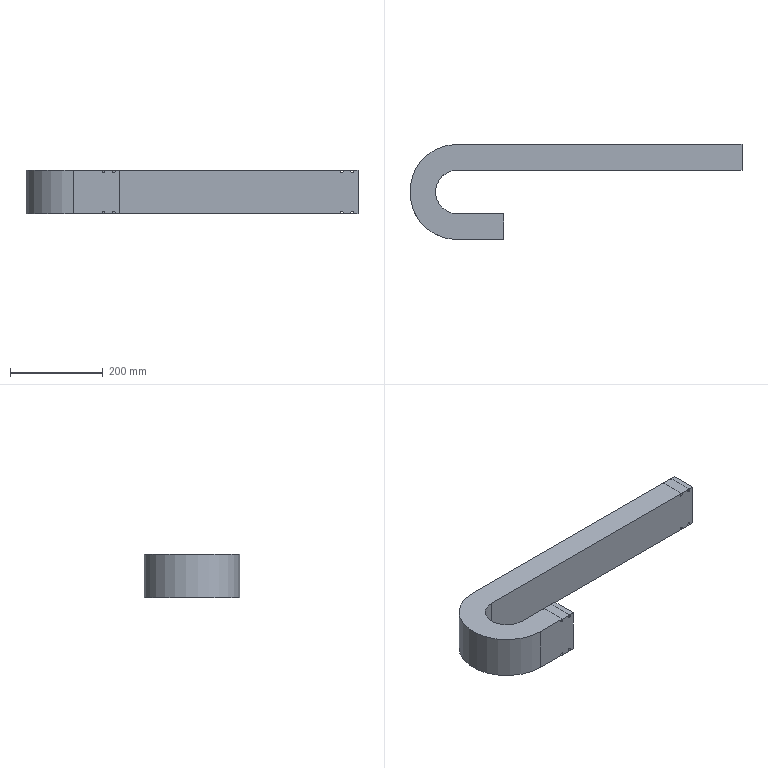Part | NX | 1 solid | 26 faces | box 718 x 206 x 95 mm | volume 1837118 mm3 | plane 14 | cylinder 12 | commonest cylinder face diameters 5.8 x8 94 x1 105 x1 195 x1 206 x1
STEP:
#1=CARTESIAN_POINT('',(0.,22.5,37.5));
#2=VERTEX_POINT('',#1);
#3=CARTESIAN_POINT('',(0.,22.5,-37.5));
#4=VERTEX_POINT('',#3);
#5=CARTESIAN_POINT('',(0.,22.5,37.5));
#6=DIRECTION('',(0.,0.,-1.));
#7=VECTOR('',#6,1000.);
#8=LINE('',#5,#7);
#9=EDGE_CURVE('',#2,#4,#8,.T.);
#10=ORIENTED_EDGE('',*,*,#9,.T.);
#11=CARTESIAN_POINT('',(100.,22.5,-37.5));
#12=VERTEX_POINT('',#11);
#13=CARTESIAN_POINT('',(0.,22.5,-37.5));
#14=DIRECTION('',(1.,0.,0.));
#15=VECTOR('',#14,1000.);
#16=LINE('',#13,#15);
#17=EDGE_CURVE('',#4,#12,#16,.T.);
#18=ORIENTED_EDGE('',*,*,#17,.T.);
#19=CARTESIAN_POINT('',(100.,22.5,37.5));
#20=VERTEX_POINT('',#19);
#21=CARTESIAN_POINT('',(100.,22.5,37.5));
#22=DIRECTION('',(0.,0.,-1.));
#23=VECTOR('',#22,1000.);
#24=LINE('',#21,#23);
#25=EDGE_CURVE('',#20,#12,#24,.T.);
#26=ORIENTED_EDGE('',*,*,#25,.F.);
#27=CARTESIAN_POINT('',(0.,22.5,37.5));
#28=DIRECTION('',(1.,0.,0.));
#29=VECTOR('',#28,1000.);
#30=LINE('',#27,#29);
#31=EDGE_CURVE('',#2,#20,#30,.T.);
#32=ORIENTED_EDGE('',*,*,#31,.F.);
#33=EDGE_LOOP('',(#10,#18,#26,#32));
#34=FACE_BOUND('',#33,.T.);
#35=CARTESIAN_POINT('',(0.,22.5,37.5));
#36=DIRECTION('',(0.,-1.,0.));
#37=DIRECTION('',(0.,0.,-1.));
#38=AXIS2_PLACEMENT_3D('',#35,#36,#37);
#39=PLANE('',#38);
#40=ADVANCED_FACE('',(#34),#39,.T.);
#41=CARTESIAN_POINT('',(0.,-22.5,-37.5));
#42=VERTEX_POINT('',#41);
#43=CARTESIAN_POINT('',(0.,-22.5,37.5));
#44=VERTEX_POINT('',#43);
#45=CARTESIAN_POINT('',(0.,-22.5,37.5));
#46=DIRECTION('',(0.,0.,1.));
#47=VECTOR('',#46,1000.);
#48=LINE('',#45,#47);
#49=EDGE_CURVE('',#42,#44,#48,.T.);
#50=ORIENTED_EDGE('',*,*,#49,.T.);
#51=CARTESIAN_POINT('',(100.,-22.5,37.5));
#52=VERTEX_POINT('',#51);
#53=CARTESIAN_POINT('',(0.,-22.5,37.5));
#54=DIRECTION('',(1.,0.,0.));
#55=VECTOR('',#54,1000.);
#56=LINE('',#53,#55);
#57=EDGE_CURVE('',#44,#52,#56,.T.);
#58=ORIENTED_EDGE('',*,*,#57,.T.);
#59=CARTESIAN_POINT('',(100.,-22.5,-37.5));
#60=VERTEX_POINT('',#59);
#61=CARTESIAN_POINT('',(100.,-22.5,37.5));
#62=DIRECTION('',(0.,0.,1.));
#63=VECTOR('',#62,1000.);
#64=LINE('',#61,#63);
#65=EDGE_CURVE('',#60,#52,#64,.T.);
#66=ORIENTED_EDGE('',*,*,#65,.F.);
#67=CARTESIAN_POINT('',(0.,-22.5,-37.5));
#68=DIRECTION('',(1.,0.,0.));
#69=VECTOR('',#68,1000.);
#70=LINE('',#67,#69);
#71=EDGE_CURVE('',#42,#60,#70,.T.);
#72=ORIENTED_EDGE('',*,*,#71,.F.);
#73=EDGE_LOOP('',(#50,#58,#66,#72));
#74=FACE_BOUND('',#73,.T.);
#75=CARTESIAN_POINT('',(0.,-22.5,37.5));
#76=DIRECTION('',(0.,1.,0.));
#77=DIRECTION('',(0.,0.,1.));
#78=AXIS2_PLACEMENT_3D('',#75,#76,#77);
#79=PLANE('',#78);
#80=ADVANCED_FACE('',(#74),#79,.T.);
#81=CARTESIAN_POINT('',(65.,28.,47.4));
#82=VERTEX_POINT('',#81);
#83=CARTESIAN_POINT('',(65.,28.,44.5));
#84=DIRECTION('',(0.,1.,0.));
#85=DIRECTION('',(0.,0.,1.));
#86=AXIS2_PLACEMENT_3D('',#83,#84,#85);
#87=CIRCLE('',#86,2.9);
#88=EDGE_CURVE('',#82,#82,#87,.T.);
#89=ORIENTED_EDGE('',*,*,#88,.F.);
#90=EDGE_LOOP('',(#89));
#91=FACE_BOUND('',#90,.T.);
#92=CARTESIAN_POINT('',(65.,28.,-41.6));
#93=VERTEX_POINT('',#92);
#94=CARTESIAN_POINT('',(65.,28.,-44.5));
#95=DIRECTION('',(0.,1.,0.));
#96=DIRECTION('',(0.,0.,1.));
#97=AXIS2_PLACEMENT_3D('',#94,#95,#96);
#98=CIRCLE('',#97,2.9);
#99=EDGE_CURVE('',#93,#93,#98,.T.);
#100=ORIENTED_EDGE('',*,*,#99,.F.);
#101=EDGE_LOOP('',(#100));
#102=FACE_BOUND('',#101,.T.);
#103=CARTESIAN_POINT('',(87.5,28.,41.6));
#104=VERTEX_POINT('',#103);
#105=CARTESIAN_POINT('',(87.5,28.,44.5));
#106=DIRECTION('',(0.,1.,0.));
#107=DIRECTION('',(0.,0.,-1.));
#108=AXIS2_PLACEMENT_3D('',#105,#106,#107);
#109=CIRCLE('',#108,2.9);
#110=EDGE_CURVE('',#104,#104,#109,.T.);
#111=ORIENTED_EDGE('',*,*,#110,.F.);
#112=EDGE_LOOP('',(#111));
#113=FACE_BOUND('',#112,.T.);
#114=CARTESIAN_POINT('',(87.5,28.,-41.6));
#115=VERTEX_POINT('',#114);
#116=CARTESIAN_POINT('',(87.5,28.,-44.5));
#117=DIRECTION('',(0.,1.,0.));
#118=DIRECTION('',(0.,0.,1.));
#119=AXIS2_PLACEMENT_3D('',#116,#117,#118);
#120=CIRCLE('',#119,2.9);
#121=EDGE_CURVE('',#115,#115,#120,.T.);
#122=ORIENTED_EDGE('',*,*,#121,.F.);
#123=EDGE_LOOP('',(#122));
#124=FACE_BOUND('',#123,.T.);
#125=CARTESIAN_POINT('',(0.,28.,47.5));
#126=VERTEX_POINT('',#125);
#127=CARTESIAN_POINT('',(0.,28.,-47.5));
#128=VERTEX_POINT('',#127);
#129=CARTESIAN_POINT('',(0.,28.,47.5));
#130=DIRECTION('',(0.,0.,-1.));
#131=VECTOR('',#130,1000.);
#132=LINE('',#129,#131);
#133=EDGE_CURVE('',#126,#128,#132,.T.);
#134=ORIENTED_EDGE('',*,*,#133,.F.);
#135=CARTESIAN_POINT('',(100.,28.,47.5));
#136=VERTEX_POINT('',#135);
#137=CARTESIAN_POINT('',(0.,28.,47.5));
#138=DIRECTION('',(1.,0.,0.));
#139=VECTOR('',#138,1000.);
#140=LINE('',#137,#139);
#141=EDGE_CURVE('',#126,#136,#140,.T.);
#142=ORIENTED_EDGE('',*,*,#141,.T.);
#143=CARTESIAN_POINT('',(100.,28.,-47.5));
#144=VERTEX_POINT('',#143);
#145=CARTESIAN_POINT('',(100.,28.,47.5));
#146=DIRECTION('',(0.,0.,-1.));
#147=VECTOR('',#146,1000.);
#148=LINE('',#145,#147);
#149=EDGE_CURVE('',#136,#144,#148,.T.);
#150=ORIENTED_EDGE('',*,*,#149,.T.);
#151=CARTESIAN_POINT('',(0.,28.,-47.5));
#152=DIRECTION('',(1.,0.,0.));
#153=VECTOR('',#152,1000.);
#154=LINE('',#151,#153);
#155=EDGE_CURVE('',#128,#144,#154,.T.);
#156=ORIENTED_EDGE('',*,*,#155,.F.);
#157=EDGE_LOOP('',(#134,#142,#150,#156));
#158=FACE_BOUND('',#157,.T.);
#159=CARTESIAN_POINT('',(0.,28.,47.5));
#160=DIRECTION('',(0.,-1.,0.));
#161=DIRECTION('',(0.,0.,-1.));
#162=AXIS2_PLACEMENT_3D('',#159,#160,#161);
#163=PLANE('',#162);
#164=ADVANCED_FACE('',(#91,#102,#113,#124,#158),#163,.F.);
#165=CARTESIAN_POINT('',(65.,-28.,47.4));
#166=VERTEX_POINT('',#165);
#167=CARTESIAN_POINT('',(65.,-28.,44.5));
#168=DIRECTION('',(0.,1.,0.));
#169=DIRECTION('',(0.,0.,1.));
#170=AXIS2_PLACEMENT_3D('',#167,#168,#169);
#171=CIRCLE('',#170,2.9);
#172=EDGE_CURVE('',#166,#166,#171,.T.);
#173=ORIENTED_EDGE('',*,*,#172,.T.);
#174=EDGE_LOOP('',(#173));
#175=FACE_BOUND('',#174,.T.);
#176=CARTESIAN_POINT('',(65.,-28.,-41.6));
#177=VERTEX_POINT('',#176);
#178=CARTESIAN_POINT('',(65.,-28.,-44.5));
#179=DIRECTION('',(0.,1.,0.));
#180=DIRECTION('',(0.,0.,1.));
#181=AXIS2_PLACEMENT_3D('',#178,#179,#180);
#182=CIRCLE('',#181,2.9);
#183=EDGE_CURVE('',#177,#177,#182,.T.);
#184=ORIENTED_EDGE('',*,*,#183,.T.);
#185=EDGE_LOOP('',(#184));
#186=FACE_BOUND('',#185,.T.);
#187=CARTESIAN_POINT('',(87.5,-28.,41.6));
#188=VERTEX_POINT('',#187);
#189=CARTESIAN_POINT('',(87.5,-28.,44.5));
#190=DIRECTION('',(0.,1.,0.));
#191=DIRECTION('',(0.,0.,-1.));
#192=AXIS2_PLACEMENT_3D('',#189,#190,#191);
#193=CIRCLE('',#192,2.9);
#194=EDGE_CURVE('',#188,#188,#193,.T.);
#195=ORIENTED_EDGE('',*,*,#194,.T.);
#196=EDGE_LOOP('',(#195));
#197=FACE_BOUND('',#196,.T.);
#198=CARTESIAN_POINT('',(87.5,-28.,-41.6));
#199=VERTEX_POINT('',#198);
#200=CARTESIAN_POINT('',(87.5,-28.,-44.5));
#201=DIRECTION('',(0.,1.,0.));
#202=DIRECTION('',(0.,0.,1.));
#203=AXIS2_PLACEMENT_3D('',#200,#201,#202);
#204=CIRCLE('',#203,2.9);
#205=EDGE_CURVE('',#199,#199,#204,.T.);
#206=ORIENTED_EDGE('',*,*,#205,.T.);
#207=EDGE_LOOP('',(#206));
#208=FACE_BOUND('',#207,.T.);
#209=CARTESIAN_POINT('',(0.,-28.,-47.5));
#210=VERTEX_POINT('',#209);
#211=CARTESIAN_POINT('',(0.,-28.,47.5));
#212=VERTEX_POINT('',#211);
#213=CARTESIAN_POINT('',(0.,-28.,47.5));
#214=DIRECTION('',(0.,0.,1.));
#215=VECTOR('',#214,1000.);
#216=LINE('',#213,#215);
#217=EDGE_CURVE('',#210,#212,#216,.T.);
#218=ORIENTED_EDGE('',*,*,#217,.F.);
#219=CARTESIAN_POINT('',(100.,-28.,-47.5));
#220=VERTEX_POINT('',#219);
#221=CARTESIAN_POINT('',(0.,-28.,-47.5));
#222=DIRECTION('',(1.,0.,0.));
#223=VECTOR('',#222,1000.);
#224=LINE('',#221,#223);
#225=EDGE_CURVE('',#210,#220,#224,.T.);
#226=ORIENTED_EDGE('',*,*,#225,.T.);
#227=CARTESIAN_POINT('',(100.,-28.,47.5));
#228=VERTEX_POINT('',#227);
#229=CARTESIAN_POINT('',(100.,-28.,47.5));
#230=DIRECTION('',(0.,0.,1.));
#231=VECTOR('',#230,1000.);
#232=LINE('',#229,#231);
#233=EDGE_CURVE('',#220,#228,#232,.T.);
#234=ORIENTED_EDGE('',*,*,#233,.T.);
#235=CARTESIAN_POINT('',(0.,-28.,47.5));
#236=DIRECTION('',(1.,0.,0.));
#237=VECTOR('',#236,1000.);
#238=LINE('',#235,#237);
#239=EDGE_CURVE('',#212,#228,#238,.T.);
#240=ORIENTED_EDGE('',*,*,#239,.F.);
#241=EDGE_LOOP('',(#218,#226,#234,#240));
#242=FACE_BOUND('',#241,.T.);
#243=CARTESIAN_POINT('',(0.,-28.,47.5));
#244=DIRECTION('',(0.,1.,0.));
#245=DIRECTION('',(0.,0.,1.));
#246=AXIS2_PLACEMENT_3D('',#243,#244,#245);
#247=PLANE('',#246);
#248=ADVANCED_FACE('',(#175,#186,#197,#208,#242),#247,.F.);
#249=CARTESIAN_POINT('',(0.,127.5,37.5));
#250=VERTEX_POINT('',#249);
#251=CARTESIAN_POINT('',(0.,127.5,-37.5));
#252=VERTEX_POINT('',#251);
#253=CARTESIAN_POINT('',(0.,127.5,37.5));
#254=DIRECTION('',(0.,0.,-1.));
#255=VECTOR('',#254,1000.);
#256=LINE('',#253,#255);
#257=EDGE_CURVE('',#250,#252,#256,.T.);
#258=ORIENTED_EDGE('',*,*,#257,.T.);
#259=CARTESIAN_POINT('',(0.,75.,-37.5));
#260=DIRECTION('',(0.,0.,1.));
#261=DIRECTION('',(1.,0.,0.));
#262=AXIS2_PLACEMENT_3D('',#259,#260,#261);
#263=CIRCLE('',#262,52.5);
#264=EDGE_CURVE('',#252,#4,#263,.T.);
#265=ORIENTED_EDGE('',*,*,#264,.T.);
#266=ORIENTED_EDGE('',*,*,#9,.F.);
#267=CARTESIAN_POINT('',(0.,75.,37.5));
#268=DIRECTION('',(0.,0.,1.));
#269=DIRECTION('',(1.,0.,0.));
#270=AXIS2_PLACEMENT_3D('',#267,#268,#269);
#271=CIRCLE('',#270,52.5);
#272=EDGE_CURVE('',#250,#2,#271,.T.);
#273=ORIENTED_EDGE('',*,*,#272,.F.);
#274=EDGE_LOOP('',(#258,#265,#266,#273));
#275=FACE_BOUND('',#274,.T.);
#276=CARTESIAN_POINT('',(0.,75.,0.));
#277=DIRECTION('',(0.,0.,1.));
#278=DIRECTION('',(1.,0.,0.));
#279=AXIS2_PLACEMENT_3D('',#276,#277,#278);
#280=CYLINDRICAL_SURFACE('',#279,52.5);
#281=ADVANCED_FACE('',(#275),#280,.T.);
#282=CARTESIAN_POINT('',(0.,172.5,-37.5));
#283=VERTEX_POINT('',#282);
#284=CARTESIAN_POINT('',(0.,172.5,37.5));
#285=VERTEX_POINT('',#284);
#286=CARTESIAN_POINT('',(0.,172.5,37.5));
#287=DIRECTION('',(0.,0.,1.));
#288=VECTOR('',#287,1000.);
#289=LINE('',#286,#288);
#290=EDGE_CURVE('',#283,#285,#289,.T.);
#291=ORIENTED_EDGE('',*,*,#290,.T.);
#292=CARTESIAN_POINT('',(0.,75.,37.5));
#293=DIRECTION('',(0.,0.,1.));
#294=DIRECTION('',(1.,0.,0.));
#295=AXIS2_PLACEMENT_3D('',#292,#293,#294);
#296=CIRCLE('',#295,97.5);
#297=EDGE_CURVE('',#285,#44,#296,.T.);
#298=ORIENTED_EDGE('',*,*,#297,.T.);
#299=ORIENTED_EDGE('',*,*,#49,.F.);
#300=CARTESIAN_POINT('',(0.,75.,-37.5));
#301=DIRECTION('',(0.,0.,1.));
#302=DIRECTION('',(1.,0.,0.));
#303=AXIS2_PLACEMENT_3D('',#300,#301,#302);
#304=CIRCLE('',#303,97.5);
#305=EDGE_CURVE('',#283,#42,#304,.T.);
#306=ORIENTED_EDGE('',*,*,#305,.F.);
#307=EDGE_LOOP('',(#291,#298,#299,#306));
#308=FACE_BOUND('',#307,.T.);
#309=CARTESIAN_POINT('',(0.,75.,0.));
#310=DIRECTION('',(0.,0.,1.));
#311=DIRECTION('',(1.,0.,0.));
#312=AXIS2_PLACEMENT_3D('',#309,#310,#311);
#313=CYLINDRICAL_SURFACE('',#312,97.5);
#314=ADVANCED_FACE('',(#308),#313,.F.);
#315=CARTESIAN_POINT('',(0.,122.,47.5));
#316=VERTEX_POINT('',#315);
#317=CARTESIAN_POINT('',(0.,122.,-47.5));
#318=VERTEX_POINT('',#317);
#319=CARTESIAN_POINT('',(0.,122.,47.5));
#320=DIRECTION('',(0.,0.,-1.));
#321=VECTOR('',#320,1000.);
#322=LINE('',#319,#321);
#323=EDGE_CURVE('',#316,#318,#322,.T.);
#324=ORIENTED_EDGE('',*,*,#323,.F.);
#325=CARTESIAN_POINT('',(0.,75.,47.5));
#326=DIRECTION('',(0.,0.,1.));
#327=DIRECTION('',(1.,0.,0.));
#328=AXIS2_PLACEMENT_3D('',#325,#326,#327);
#329=CIRCLE('',#328,47.);
#330=EDGE_CURVE('',#316,#126,#329,.T.);
#331=ORIENTED_EDGE('',*,*,#330,.T.);
#332=ORIENTED_EDGE('',*,*,#133,.T.);
#333=CARTESIAN_POINT('',(0.,75.,-47.5));
#334=DIRECTION('',(0.,0.,1.));
#335=DIRECTION('',(1.,0.,0.));
#336=AXIS2_PLACEMENT_3D('',#333,#334,#335);
#337=CIRCLE('',#336,47.);
#338=EDGE_CURVE('',#318,#128,#337,.T.);
#339=ORIENTED_EDGE('',*,*,#338,.F.);
#340=EDGE_LOOP('',(#324,#331,#332,#339));
#341=FACE_BOUND('',#340,.T.);
#342=CARTESIAN_POINT('',(0.,75.,0.));
#343=DIRECTION('',(0.,0.,1.));
#344=DIRECTION('',(1.,0.,0.));
#345=AXIS2_PLACEMENT_3D('',#342,#343,#344);
#346=CYLINDRICAL_SURFACE('',#345,47.);
#347=ADVANCED_FACE('',(#341),#346,.F.);
#348=CARTESIAN_POINT('',(0.,178.,-47.5));
#349=VERTEX_POINT('',#348);
#350=CARTESIAN_POINT('',(0.,178.,47.5));
#351=VERTEX_POINT('',#350);
#352=CARTESIAN_POINT('',(0.,178.,47.5));
#353=DIRECTION('',(0.,0.,1.));
#354=VECTOR('',#353,1000.);
#355=LINE('',#352,#354);
#356=EDGE_CURVE('',#349,#351,#355,.T.);
#357=ORIENTED_EDGE('',*,*,#356,.F.);
#358=CARTESIAN_POINT('',(0.,75.,-47.5));
#359=DIRECTION('',(0.,0.,1.));
#360=DIRECTION('',(1.,0.,0.));
#361=AXIS2_PLACEMENT_3D('',#358,#359,#360);
#362=CIRCLE('',#361,103.);
#363=EDGE_CURVE('',#349,#210,#362,.T.);
#364=ORIENTED_EDGE('',*,*,#363,.T.);
#365=ORIENTED_EDGE('',*,*,#217,.T.);
#366=CARTESIAN_POINT('',(0.,75.,47.5));
#367=DIRECTION('',(0.,0.,1.));
#368=DIRECTION('',(1.,0.,0.));
#369=AXIS2_PLACEMENT_3D('',#366,#367,#368);
#370=CIRCLE('',#369,103.);
#371=EDGE_CURVE('',#351,#212,#370,.T.);
#372=ORIENTED_EDGE('',*,*,#371,.F.);
#373=EDGE_LOOP('',(#357,#364,#365,#372));
#374=FACE_BOUND('',#373,.T.);
#375=CARTESIAN_POINT('',(0.,75.,0.));
#376=DIRECTION('',(0.,0.,1.));
#377=DIRECTION('',(1.,0.,0.));
#378=AXIS2_PLACEMENT_3D('',#375,#376,#377);
#379=CYLINDRICAL_SURFACE('',#378,103.);
#380=ADVANCED_FACE('',(#374),#379,.T.);
#381=CARTESIAN_POINT('',(615.,172.5,37.5));
#382=VERTEX_POINT('',#381);
#383=CARTESIAN_POINT('',(615.,127.5,37.5));
#384=VERTEX_POINT('',#383);
#385=CARTESIAN_POINT('',(615.,127.5,37.5));
#386=DIRECTION('',(0.,-1.,0.));
#387=VECTOR('',#386,1000.);
#388=LINE('',#385,#387);
#389=EDGE_CURVE('',#382,#384,#388,.T.);
#390=ORIENTED_EDGE('',*,*,#389,.T.);
#391=CARTESIAN_POINT('',(0.,127.5,37.5));
#392=DIRECTION('',(1.,0.,0.));
#393=VECTOR('',#392,1000.);
#394=LINE('',#391,#393);
#395=EDGE_CURVE('',#250,#384,#394,.T.);
#396=ORIENTED_EDGE('',*,*,#395,.F.);
#397=ORIENTED_EDGE('',*,*,#272,.T.);
#398=ORIENTED_EDGE('',*,*,#31,.T.);
#399=CARTESIAN_POINT('',(100.,22.5,37.5));
#400=DIRECTION('',(0.,1.,0.));
#401=VECTOR('',#400,1000.);
#402=LINE('',#399,#401);
#403=EDGE_CURVE('',#52,#20,#402,.T.);
#404=ORIENTED_EDGE('',*,*,#403,.F.);
#405=ORIENTED_EDGE('',*,*,#57,.F.);
#406=ORIENTED_EDGE('',*,*,#297,.F.);
#407=CARTESIAN_POINT('',(0.,172.5,37.5));
#408=DIRECTION('',(1.,0.,0.));
#409=VECTOR('',#408,1000.);
#410=LINE('',#407,#409);
#411=EDGE_CURVE('',#285,#382,#410,.T.);
#412=ORIENTED_EDGE('',*,*,#411,.T.);
#413=EDGE_LOOP('',(#390,#396,#397,#398,#404,#405,#406,#412));
#414=FACE_BOUND('',#413,.T.);
#415=CARTESIAN_POINT('',(0.,127.5,37.5));
#416=DIRECTION('',(0.,0.,1.));
#417=DIRECTION('',(1.,0.,0.));
#418=AXIS2_PLACEMENT_3D('',#415,#416,#417);
#419=PLANE('',#418);
#420=ADVANCED_FACE('',(#414),#419,.F.);
#421=CARTESIAN_POINT('',(615.,127.5,-37.5));
#422=VERTEX_POINT('',#421);
#423=CARTESIAN_POINT('',(615.,127.5,37.5));
#424=DIRECTION('',(0.,0.,-1.));
#425=VECTOR('',#424,1000.);
#426=LINE('',#423,#425);
#427=EDGE_CURVE('',#384,#422,#426,.T.);
#428=ORIENTED_EDGE('',*,*,#427,.T.);
#429=CARTESIAN_POINT('',(0.,127.5,-37.5));
#430=DIRECTION('',(1.,0.,0.));
#431=VECTOR('',#430,1000.);
#432=LINE('',#429,#431);
#433=EDGE_CURVE('',#252,#422,#432,.T.);
#434=ORIENTED_EDGE('',*,*,#433,.F.);
#435=ORIENTED_EDGE('',*,*,#257,.F.);
#436=ORIENTED_EDGE('',*,*,#395,.T.);
#437=EDGE_LOOP('',(#428,#434,#435,#436));
#438=FACE_BOUND('',#437,.T.);
#439=CARTESIAN_POINT('',(0.,127.5,37.5));
#440=DIRECTION('',(0.,-1.,0.));
#441=DIRECTION('',(1.,0.,0.));
#442=AXIS2_PLACEMENT_3D('',#439,#440,#441);
#443=PLANE('',#442);
#444=ADVANCED_FACE('',(#438),#443,.F.);
#445=CARTESIAN_POINT('',(615.,172.5,-37.5));
#446=VERTEX_POINT('',#445);
#447=CARTESIAN_POINT('',(615.,127.5,-37.5));
#448=DIRECTION('',(0.,1.,0.));
#449=VECTOR('',#448,1000.);
#450=LINE('',#447,#449);
#451=EDGE_CURVE('',#422,#446,#450,.T.);
#452=ORIENTED_EDGE('',*,*,#451,.T.);
#453=CARTESIAN_POINT('',(0.,172.5,-37.5));
#454=DIRECTION('',(1.,0.,0.));
#455=VECTOR('',#454,1000.);
#456=LINE('',#453,#455);
#457=EDGE_CURVE('',#283,#446,#456,.T.);
#458=ORIENTED_EDGE('',*,*,#457,.F.);
#459=ORIENTED_EDGE('',*,*,#305,.T.);
#460=ORIENTED_EDGE('',*,*,#71,.T.);
#461=CARTESIAN_POINT('',(100.,22.5,-37.5));
#462=DIRECTION('',(0.,-1.,0.));
#463=VECTOR('',#462,1000.);
#464=LINE('',#461,#463);
#465=EDGE_CURVE('',#12,#60,#464,.T.);
#466=ORIENTED_EDGE('',*,*,#465,.F.);
#467=ORIENTED_EDGE('',*,*,#17,.F.);
#468=ORIENTED_EDGE('',*,*,#264,.F.);
#469=ORIENTED_EDGE('',*,*,#433,.T.);
#470=EDGE_LOOP('',(#452,#458,#459,#460,#466,#467,#468,#469));
#471=FACE_BOUND('',#470,.T.);
#472=CARTESIAN_POINT('',(0.,127.5,-37.5));
#473=DIRECTION('',(0.,0.,-1.));
#474=DIRECTION('',(-1.,0.,0.));
#475=AXIS2_PLACEMENT_3D('',#472,#473,#474);
#476=PLANE('',#475);
#477=ADVANCED_FACE('',(#471),#476,.F.);
#478=CARTESIAN_POINT('',(615.,122.,-47.5));
#479=VERTEX_POINT('',#478);
#480=CARTESIAN_POINT('',(615.,178.,-47.5));
#481=VERTEX_POINT('',#480);
#482=CARTESIAN_POINT('',(615.,122.,-47.5));
#483=DIRECTION('',(0.,1.,0.));
#484=VECTOR('',#483,1000.);
#485=LINE('',#482,#484);
#486=EDGE_CURVE('',#479,#481,#485,.T.);
#487=ORIENTED_EDGE('',*,*,#486,.F.);
#488=CARTESIAN_POINT('',(0.,122.,-47.5));
#489=DIRECTION('',(1.,0.,0.));
#490=VECTOR('',#489,1000.);
#491=LINE('',#488,#490);
#492=EDGE_CURVE('',#318,#479,#491,.T.);
#493=ORIENTED_EDGE('',*,*,#492,.F.);
#494=ORIENTED_EDGE('',*,*,#338,.T.);
#495=ORIENTED_EDGE('',*,*,#155,.T.);
#496=CARTESIAN_POINT('',(100.,28.,-47.5));
#497=DIRECTION('',(0.,-1.,0.));
#498=VECTOR('',#497,1000.);
#499=LINE('',#496,#498);
#500=EDGE_CURVE('',#144,#220,#499,.T.);
#501=ORIENTED_EDGE('',*,*,#500,.T.);
#502=ORIENTED_EDGE('',*,*,#225,.F.);
#503=ORIENTED_EDGE('',*,*,#363,.F.);
#504=CARTESIAN_POINT('',(0.,178.,-47.5));
#505=DIRECTION('',(1.,0.,0.));
#506=VECTOR('',#505,1000.);
#507=LINE('',#504,#506);
#508=EDGE_CURVE('',#349,#481,#507,.T.);
#509=ORIENTED_EDGE('',*,*,#508,.T.);
#510=EDGE_LOOP('',(#487,#493,#494,#495,#501,#502,#503,#509));
#511=FACE_BOUND('',#510,.T.);
#512=CARTESIAN_POINT('',(0.,122.,-47.5));
#513=DIRECTION('',(0.,0.,-1.));
#514=DIRECTION('',(-1.,0.,0.));
#515=AXIS2_PLACEMENT_3D('',#512,#513,#514);
#516=PLANE('',#515);
#517=ADVANCED_FACE('',(#511),#516,.T.);
#518=CARTESIAN_POINT('',(582.9,122.,44.5));
#519=VERTEX_POINT('',#518);
#520=CARTESIAN_POINT('',(580.,122.,44.5));
#521=DIRECTION('',(0.,-1.,0.));
#522=DIRECTION('',(1.,0.,0.));
#523=AXIS2_PLACEMENT_3D('',#520,#521,#522);
#524=CIRCLE('',#523,2.9);
#525=EDGE_CURVE('',#519,#519,#524,.T.);
#526=ORIENTED_EDGE('',*,*,#525,.F.);
#527=EDGE_LOOP('',(#526));
#528=FACE_BOUND('',#527,.T.);
#529=CARTESIAN_POINT('',(582.9,122.,-44.5));
#530=VERTEX_POINT('',#529);
#531=CARTESIAN_POINT('',(580.,122.,-44.5));
#532=DIRECTION('',(0.,-1.,0.));
#533=DIRECTION('',(1.,0.,0.));
#534=AXIS2_PLACEMENT_3D('',#531,#532,#533);
#535=CIRCLE('',#534,2.9);
#536=EDGE_CURVE('',#530,#530,#535,.T.);
#537=ORIENTED_EDGE('',*,*,#536,.F.);
#538=EDGE_LOOP('',(#537));
#539=FACE_BOUND('',#538,.T.);
#540=CARTESIAN_POINT('',(605.4,122.,44.5));
#541=VERTEX_POINT('',#540);
#542=CARTESIAN_POINT('',(602.5,122.,44.5));
#543=DIRECTION('',(0.,-1.,0.));
#544=DIRECTION('',(1.,0.,0.));
#545=AXIS2_PLACEMENT_3D('',#542,#543,#544);
#546=CIRCLE('',#545,2.9);
#547=EDGE_CURVE('',#541,#541,#546,.T.);
#548=ORIENTED_EDGE('',*,*,#547,.F.);
#549=EDGE_LOOP('',(#548));
#550=FACE_BOUND('',#549,.T.);
#551=CARTESIAN_POINT('',(605.4,122.,-44.5));
#552=VERTEX_POINT('',#551);
#553=CARTESIAN_POINT('',(602.5,122.,-44.5));
#554=DIRECTION('',(0.,-1.,0.));
#555=DIRECTION('',(1.,0.,0.));
#556=AXIS2_PLACEMENT_3D('',#553,#554,#555);
#557=CIRCLE('',#556,2.9);
#558=EDGE_CURVE('',#552,#552,#557,.T.);
#559=ORIENTED_EDGE('',*,*,#558,.F.);
#560=EDGE_LOOP('',(#559));
#561=FACE_BOUND('',#560,.T.);
#562=CARTESIAN_POINT('',(615.,122.,47.5));
#563=VERTEX_POINT('',#562);
#564=CARTESIAN_POINT('',(615.,122.,47.5));
#565=DIRECTION('',(0.,0.,-1.));
#566=VECTOR('',#565,1000.);
#567=LINE('',#564,#566);
#568=EDGE_CURVE('',#563,#479,#567,.T.);
#569=ORIENTED_EDGE('',*,*,#568,.F.);
#570=CARTESIAN_POINT('',(0.,122.,47.5));
#571=DIRECTION('',(1.,0.,0.));
#572=VECTOR('',#571,1000.);
#573=LINE('',#570,#572);
#574=EDGE_CURVE('',#316,#563,#573,.T.);
#575=ORIENTED_EDGE('',*,*,#574,.F.);
#576=ORIENTED_EDGE('',*,*,#323,.T.);
#577=ORIENTED_EDGE('',*,*,#492,.T.);
#578=EDGE_LOOP('',(#569,#575,#576,#577));
#579=FACE_BOUND('',#578,.T.);
#580=CARTESIAN_POINT('',(0.,122.,47.5));
#581=DIRECTION('',(0.,-1.,0.));
#582=DIRECTION('',(1.,0.,0.));
#583=AXIS2_PLACEMENT_3D('',#580,#581,#582);
#584=PLANE('',#583);
#585=ADVANCED_FACE('',(#528,#539,#550,#561,#579),#584,.T.);
#586=CARTESIAN_POINT('',(615.,178.,47.5));
#587=VERTEX_POINT('',#586);
#588=CARTESIAN_POINT('',(615.,122.,47.5));
#589=DIRECTION('',(0.,-1.,0.));
#590=VECTOR('',#589,1000.);
#591=LINE('',#588,#590);
#592=EDGE_CURVE('',#587,#563,#591,.T.);
#593=ORIENTED_EDGE('',*,*,#592,.F.);
#594=CARTESIAN_POINT('',(0.,178.,47.5));
#595=DIRECTION('',(1.,0.,0.));
#596=VECTOR('',#595,1000.);
#597=LINE('',#594,#596);
#598=EDGE_CURVE('',#351,#587,#597,.T.);
#599=ORIENTED_EDGE('',*,*,#598,.F.);
#600=ORIENTED_EDGE('',*,*,#371,.T.);
#601=ORIENTED_EDGE('',*,*,#239,.T.);
#602=CARTESIAN_POINT('',(100.,28.,47.5));
#603=DIRECTION('',(0.,1.,0.));
#604=VECTOR('',#603,1000.);
#605=LINE('',#602,#604);
#606=EDGE_CURVE('',#228,#136,#605,.T.);
#607=ORIENTED_EDGE('',*,*,#606,.T.);
#608=ORIENTED_EDGE('',*,*,#141,.F.);
#609=ORIENTED_EDGE('',*,*,#330,.F.);
#610=ORIENTED_EDGE('',*,*,#574,.T.);
#611=EDGE_LOOP('',(#593,#599,#600,#601,#607,#608,#609,#610));
#612=FACE_BOUND('',#611,.T.);
#613=CARTESIAN_POINT('',(0.,122.,47.5));
#614=DIRECTION('',(0.,0.,1.));
#615=DIRECTION('',(1.,0.,0.));
#616=AXIS2_PLACEMENT_3D('',#613,#614,#615);
#617=PLANE('',#616);
#618=ADVANCED_FACE('',(#612),#617,.T.);
#619=CARTESIAN_POINT('',(580.,178.,47.4));
#620=VERTEX_POINT('',#619);
#621=CARTESIAN_POINT('',(580.,178.,44.5));
#622=DIRECTION('',(0.,1.,0.));
#623=DIRECTION('',(0.,0.,1.));
#624=AXIS2_PLACEMENT_3D('',#621,#622,#623);
#625=CIRCLE('',#624,2.9);
#626=EDGE_CURVE('',#620,#620,#625,.T.);
#627=ORIENTED_EDGE('',*,*,#626,.F.);
#628=EDGE_LOOP('',(#627));
#629=FACE_BOUND('',#628,.T.);
#630=CARTESIAN_POINT('',(580.,178.,-41.6));
#631=VERTEX_POINT('',#630);
#632=CARTESIAN_POINT('',(580.,178.,-44.5));
#633=DIRECTION('',(0.,1.,0.));
#634=DIRECTION('',(0.,0.,1.));
#635=AXIS2_PLACEMENT_3D('',#632,#633,#634);
#636=CIRCLE('',#635,2.9);
#637=EDGE_CURVE('',#631,#631,#636,.T.);
#638=ORIENTED_EDGE('',*,*,#637,.F.);
#639=EDGE_LOOP('',(#638));
#640=FACE_BOUND('',#639,.T.);
#641=CARTESIAN_POINT('',(602.5,178.,47.4));
#642=VERTEX_POINT('',#641);
#643=CARTESIAN_POINT('',(602.5,178.,44.5));
#644=DIRECTION('',(0.,1.,0.));
#645=DIRECTION('',(0.,0.,1.));
#646=AXIS2_PLACEMENT_3D('',#643,#644,#645);
#647=CIRCLE('',#646,2.9);
#648=EDGE_CURVE('',#642,#642,#647,.T.);
#649=ORIENTED_EDGE('',*,*,#648,.F.);
#650=EDGE_LOOP('',(#649));
#651=FACE_BOUND('',#650,.T.);
#652=CARTESIAN_POINT('',(602.5,178.,-41.6));
#653=VERTEX_POINT('',#652);
#654=CARTESIAN_POINT('',(602.5,178.,-44.5));
#655=DIRECTION('',(0.,1.,0.));
#656=DIRECTION('',(0.,0.,1.));
#657=AXIS2_PLACEMENT_3D('',#654,#655,#656);
#658=CIRCLE('',#657,2.9);
#659=EDGE_CURVE('',#653,#653,#658,.T.);
#660=ORIENTED_EDGE('',*,*,#659,.F.);
#661=EDGE_LOOP('',(#660));
#662=FACE_BOUND('',#661,.T.);
#663=CARTESIAN_POINT('',(615.,178.,47.5));
#664=DIRECTION('',(0.,0.,1.));
#665=VECTOR('',#664,1000.);
#666=LINE('',#663,#665);
#667=EDGE_CURVE('',#481,#587,#666,.T.);
#668=ORIENTED_EDGE('',*,*,#667,.F.);
#669=ORIENTED_EDGE('',*,*,#508,.F.);
#670=ORIENTED_EDGE('',*,*,#356,.T.);
#671=ORIENTED_EDGE('',*,*,#598,.T.);
#672=EDGE_LOOP('',(#668,#669,#670,#671));
#673=FACE_BOUND('',#672,.T.);
#674=CARTESIAN_POINT('',(0.,178.,47.5));
#675=DIRECTION('',(0.,1.,0.));
#676=DIRECTION('',(-1.,0.,0.));
#677=AXIS2_PLACEMENT_3D('',#674,#675,#676);
#678=PLANE('',#677);
#679=ADVANCED_FACE('',(#629,#640,#651,#662,#673),#678,.T.);
#680=CARTESIAN_POINT('',(615.,172.5,37.5));
#681=DIRECTION('',(0.,0.,1.));
#682=VECTOR('',#681,1000.);
#683=LINE('',#680,#682);
#684=EDGE_CURVE('',#446,#382,#683,.T.);
#685=ORIENTED_EDGE('',*,*,#684,.T.);
#686=ORIENTED_EDGE('',*,*,#411,.F.);
#687=ORIENTED_EDGE('',*,*,#290,.F.);
#688=ORIENTED_EDGE('',*,*,#457,.T.);
#689=EDGE_LOOP('',(#685,#686,#687,#688));
#690=FACE_BOUND('',#689,.T.);
#691=CARTESIAN_POINT('',(0.,172.5,37.5));
#692=DIRECTION('',(0.,1.,0.));
#693=DIRECTION('',(-1.,0.,0.));
#694=AXIS2_PLACEMENT_3D('',#691,#692,#693);
#695=PLANE('',#694);
#696=ADVANCED_FACE('',(#690),#695,.F.);
#697=ORIENTED_EDGE('',*,*,#500,.F.);
#698=ORIENTED_EDGE('',*,*,#149,.F.);
#699=ORIENTED_EDGE('',*,*,#606,.F.);
#700=ORIENTED_EDGE('',*,*,#233,.F.);
#701=EDGE_LOOP('',(#697,#698,#699,#700));
#702=FACE_BOUND('',#701,.T.);
#703=ORIENTED_EDGE('',*,*,#403,.T.);
#704=ORIENTED_EDGE('',*,*,#25,.T.);
#705=ORIENTED_EDGE('',*,*,#465,.T.);
#706=ORIENTED_EDGE('',*,*,#65,.T.);
#707=EDGE_LOOP('',(#703,#704,#705,#706));
#708=FACE_BOUND('',#707,.T.);
#709=CARTESIAN_POINT('',(100.,150.,0.));
#710=DIRECTION('',(1.,0.,0.));
#711=DIRECTION('',(0.,0.,1.));
#712=AXIS2_PLACEMENT_3D('',#709,#710,#711);
#713=PLANE('',#712);
#714=ADVANCED_FACE('',(#702,#708),#713,.T.);
#715=ORIENTED_EDGE('',*,*,#486,.T.);
#716=ORIENTED_EDGE('',*,*,#667,.T.);
#717=ORIENTED_EDGE('',*,*,#592,.T.);
#718=ORIENTED_EDGE('',*,*,#568,.T.);
#719=EDGE_LOOP('',(#715,#716,#717,#718));
#720=FACE_BOUND('',#719,.T.);
#721=ORIENTED_EDGE('',*,*,#389,.F.);
#722=ORIENTED_EDGE('',*,*,#684,.F.);
#723=ORIENTED_EDGE('',*,*,#451,.F.);
#724=ORIENTED_EDGE('',*,*,#427,.F.);
#725=EDGE_LOOP('',(#721,#722,#723,#724));
#726=FACE_BOUND('',#725,.T.);
#727=CARTESIAN_POINT('',(615.,0.,0.));
#728=DIRECTION('',(-1.,0.,0.));
#729=DIRECTION('',(0.,0.,1.));
#730=AXIS2_PLACEMENT_3D('',#727,#728,#729);
#731=PLANE('',#730);
#732=ADVANCED_FACE('',(#720,#726),#731,.F.);
#733=ORIENTED_EDGE('',*,*,#558,.T.);
#734=EDGE_LOOP('',(#733));
#735=FACE_BOUND('',#734,.T.);
#736=ORIENTED_EDGE('',*,*,#659,.T.);
#737=EDGE_LOOP('',(#736));
#738=FACE_BOUND('',#737,.T.);
#739=CARTESIAN_POINT('',(602.5,98.,-44.5));
#740=DIRECTION('',(0.,1.,0.));
#741=DIRECTION('',(0.,0.,1.));
#742=AXIS2_PLACEMENT_3D('',#739,#740,#741);
#743=CYLINDRICAL_SURFACE('',#742,2.9);
#744=ADVANCED_FACE('',(#735,#738),#743,.F.);
#745=ORIENTED_EDGE('',*,*,#547,.T.);
#746=EDGE_LOOP('',(#745));
#747=FACE_BOUND('',#746,.T.);
#748=ORIENTED_EDGE('',*,*,#648,.T.);
#749=EDGE_LOOP('',(#748));
#750=FACE_BOUND('',#749,.T.);
#751=CARTESIAN_POINT('',(602.5,98.,44.5));
#752=DIRECTION('',(0.,1.,0.));
#753=DIRECTION('',(0.,0.,1.));
#754=AXIS2_PLACEMENT_3D('',#751,#752,#753);
#755=CYLINDRICAL_SURFACE('',#754,2.9);
#756=ADVANCED_FACE('',(#747,#750),#755,.F.);
#757=ORIENTED_EDGE('',*,*,#536,.T.);
#758=EDGE_LOOP('',(#757));
#759=FACE_BOUND('',#758,.T.);
#760=ORIENTED_EDGE('',*,*,#637,.T.);
#761=EDGE_LOOP('',(#760));
#762=FACE_BOUND('',#761,.T.);
#763=CARTESIAN_POINT('',(580.,98.,-44.5));
#764=DIRECTION('',(0.,1.,0.));
#765=DIRECTION('',(0.,0.,1.));
#766=AXIS2_PLACEMENT_3D('',#763,#764,#765);
#767=CYLINDRICAL_SURFACE('',#766,2.9);
#768=ADVANCED_FACE('',(#759,#762),#767,.F.);
#769=ORIENTED_EDGE('',*,*,#525,.T.);
#770=EDGE_LOOP('',(#769));
#771=FACE_BOUND('',#770,.T.);
#772=ORIENTED_EDGE('',*,*,#626,.T.);
#773=EDGE_LOOP('',(#772));
#774=FACE_BOUND('',#773,.T.);
#775=CARTESIAN_POINT('',(580.,98.,44.5));
#776=DIRECTION('',(0.,1.,0.));
#777=DIRECTION('',(0.,0.,1.));
#778=AXIS2_PLACEMENT_3D('',#775,#776,#777);
#779=CYLINDRICAL_SURFACE('',#778,2.9);
#780=ADVANCED_FACE('',(#771,#774),#779,.F.);
#781=ORIENTED_EDGE('',*,*,#205,.F.);
#782=EDGE_LOOP('',(#781));
#783=FACE_BOUND('',#782,.T.);
#784=ORIENTED_EDGE('',*,*,#121,.T.);
#785=EDGE_LOOP('',(#784));
#786=FACE_BOUND('',#785,.T.);
#787=CARTESIAN_POINT('',(87.5,-28.,-44.5));
#788=DIRECTION('',(0.,1.,0.));
#789=DIRECTION('',(0.,0.,1.));
#790=AXIS2_PLACEMENT_3D('',#787,#788,#789);
#791=CYLINDRICAL_SURFACE('',#790,2.9);
#792=ADVANCED_FACE('',(#783,#786),#791,.F.);
#793=ORIENTED_EDGE('',*,*,#194,.F.);
#794=EDGE_LOOP('',(#793));
#795=FACE_BOUND('',#794,.T.);
#796=ORIENTED_EDGE('',*,*,#110,.T.);
#797=EDGE_LOOP('',(#796));
#798=FACE_BOUND('',#797,.T.);
#799=CARTESIAN_POINT('',(87.5,-28.,44.5));
#800=DIRECTION('',(0.,1.,0.));
#801=DIRECTION('',(0.,0.,1.));
#802=AXIS2_PLACEMENT_3D('',#799,#800,#801);
#803=CYLINDRICAL_SURFACE('',#802,2.9);
#804=ADVANCED_FACE('',(#795,#798),#803,.F.);
#805=ORIENTED_EDGE('',*,*,#183,.F.);
#806=EDGE_LOOP('',(#805));
#807=FACE_BOUND('',#806,.T.);
#808=ORIENTED_EDGE('',*,*,#99,.T.);
#809=EDGE_LOOP('',(#808));
#810=FACE_BOUND('',#809,.T.);
#811=CARTESIAN_POINT('',(65.,-28.,-44.5));
#812=DIRECTION('',(0.,1.,0.));
#813=DIRECTION('',(0.,0.,1.));
#814=AXIS2_PLACEMENT_3D('',#811,#812,#813);
#815=CYLINDRICAL_SURFACE('',#814,2.9);
#816=ADVANCED_FACE('',(#807,#810),#815,.F.);
#817=ORIENTED_EDGE('',*,*,#172,.F.);
#818=EDGE_LOOP('',(#817));
#819=FACE_BOUND('',#818,.T.);
#820=ORIENTED_EDGE('',*,*,#88,.T.);
#821=EDGE_LOOP('',(#820));
#822=FACE_BOUND('',#821,.T.);
#823=CARTESIAN_POINT('',(65.,-28.,44.5));
#824=DIRECTION('',(0.,1.,0.));
#825=DIRECTION('',(0.,0.,1.));
#826=AXIS2_PLACEMENT_3D('',#823,#824,#825);
#827=CYLINDRICAL_SURFACE('',#826,2.9);
#828=ADVANCED_FACE('',(#819,#822),#827,.F.);
#829=CLOSED_SHELL('',(#40,#80,#164,#248,#281,#314,#347,#380,#420,#444,#477,#517,#585,#618,#679,#696,#714,#732,#744,#756,#768,#780,#792,#804,#816,#828));
#830=MANIFOLD_SOLID_BREP('',#829);
#831=(LENGTH_UNIT()NAMED_UNIT(*)SI_UNIT(.MILLI.,.METRE.));
#832=UNCERTAINTY_MEASURE_WITH_UNIT(LENGTH_MEASURE(0.00001),#831,'','');
#833=(NAMED_UNIT(*)PLANE_ANGLE_UNIT()SI_UNIT($,.RADIAN.));
#834=(NAMED_UNIT(*)SI_UNIT($,.STERADIAN.)SOLID_ANGLE_UNIT());
#835=(GEOMETRIC_REPRESENTATION_CONTEXT(3)GLOBAL_UNCERTAINTY_ASSIGNED_CONTEXT((#832))GLOBAL_UNIT_ASSIGNED_CONTEXT((#831,#833,#834))REPRESENTATION_CONTEXT('',''));
#836=ADVANCED_BREP_SHAPE_REPRESENTATION('',(#830),#835);